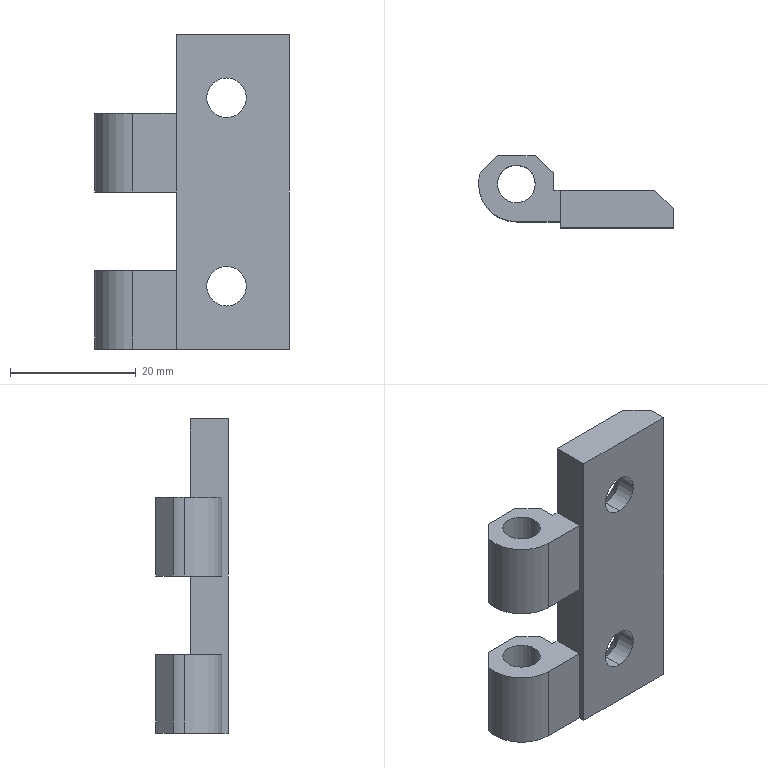Part | SolidWorks | 1 solid | 36 faces | box 31 x 11.5 x 50 mm | volume 6739 mm3 | plane 20 | cylinder 12 | cone 4 | commonest cylinder face diameters 6 x4 6.3 x4 12 x4
STEP:
#1=CARTESIAN_POINT('',(8.,3.15,-18.15));
#2=VERTEX_POINT('',#1);
#3=CARTESIAN_POINT('',(8.,3.15,-11.85));
#4=VERTEX_POINT('',#3);
#5=CARTESIAN_POINT('',(8.,3.15,-15.));
#6=DIRECTION('',(0.,1.,0.));
#7=DIRECTION('',(0.,0.,1.));
#8=AXIS2_PLACEMENT_3D('',#5,#6,#7);
#9=CIRCLE('',#8,3.15);
#10=EDGE_CURVE('',#2,#4,#9,.T.);
#11=ORIENTED_EDGE('',*,*,#10,.F.);
#12=CARTESIAN_POINT('',(8.,6.,-21.));
#13=VERTEX_POINT('',#12);
#14=CARTESIAN_POINT('',(8.,6.,-21.));
#15=DIRECTION('',(0.,0.7071,-0.7071));
#16=VECTOR('',#15,1000.);
#17=LINE('',#14,#16);
#18=EDGE_CURVE('',#2,#13,#17,.T.);
#19=ORIENTED_EDGE('',*,*,#18,.T.);
#20=CARTESIAN_POINT('',(8.,6.,-9.));
#21=VERTEX_POINT('',#20);
#22=CARTESIAN_POINT('',(8.,6.,-15.));
#23=DIRECTION('',(0.,1.,0.));
#24=DIRECTION('',(0.,0.,1.));
#25=AXIS2_PLACEMENT_3D('',#22,#23,#24);
#26=CIRCLE('',#25,6.);
#27=EDGE_CURVE('',#13,#21,#26,.T.);
#28=ORIENTED_EDGE('',*,*,#27,.T.);
#29=CARTESIAN_POINT('',(8.,6.,-9.));
#30=DIRECTION('',(0.,0.7071,0.7071));
#31=VECTOR('',#30,1000.);
#32=LINE('',#29,#31);
#33=EDGE_CURVE('',#4,#21,#32,.T.);
#34=ORIENTED_EDGE('',*,*,#33,.F.);
#35=EDGE_LOOP('',(#11,#19,#28,#34));
#36=FACE_OUTER_BOUND('',#35,.T.);
#37=CARTESIAN_POINT('',(8.,6.,-15.));
#38=DIRECTION('',(0.,1.,0.));
#39=DIRECTION('',(0.,0.,1.));
#40=AXIS2_PLACEMENT_3D('',#37,#38,#39);
#41=CONICAL_SURFACE('',#40,6.,0.7854);
#42=ADVANCED_FACE('',(#36),#41,.F.);
#43=CARTESIAN_POINT('',(8.,0.,-18.15));
#44=VERTEX_POINT('',#43);
#45=CARTESIAN_POINT('',(8.,0.,-11.85));
#46=VERTEX_POINT('',#45);
#47=CARTESIAN_POINT('',(8.,0.,-15.));
#48=DIRECTION('',(0.,1.,0.));
#49=DIRECTION('',(0.,0.,1.));
#50=AXIS2_PLACEMENT_3D('',#47,#48,#49);
#51=CIRCLE('',#50,3.15);
#52=EDGE_CURVE('',#44,#46,#51,.T.);
#53=ORIENTED_EDGE('',*,*,#52,.F.);
#54=CARTESIAN_POINT('',(8.,6.,-18.15));
#55=DIRECTION('',(0.,1.,0.));
#56=VECTOR('',#55,1000.);
#57=LINE('',#54,#56);
#58=EDGE_CURVE('',#44,#2,#57,.T.);
#59=ORIENTED_EDGE('',*,*,#58,.T.);
#60=ORIENTED_EDGE('',*,*,#10,.T.);
#61=CARTESIAN_POINT('',(8.,6.,-11.85));
#62=DIRECTION('',(0.,1.,0.));
#63=VECTOR('',#62,1000.);
#64=LINE('',#61,#63);
#65=EDGE_CURVE('',#46,#4,#64,.T.);
#66=ORIENTED_EDGE('',*,*,#65,.F.);
#67=EDGE_LOOP('',(#53,#59,#60,#66));
#68=FACE_OUTER_BOUND('',#67,.T.);
#69=CARTESIAN_POINT('',(8.,6.,-15.));
#70=DIRECTION('',(0.,1.,0.));
#71=DIRECTION('',(0.,0.,1.));
#72=AXIS2_PLACEMENT_3D('',#69,#70,#71);
#73=CYLINDRICAL_SURFACE('',#72,3.15);
#74=ADVANCED_FACE('',(#68),#73,.F.);
#75=CARTESIAN_POINT('',(8.,3.15,11.85));
#76=VERTEX_POINT('',#75);
#77=CARTESIAN_POINT('',(8.,3.15,18.15));
#78=VERTEX_POINT('',#77);
#79=CARTESIAN_POINT('',(8.,3.15,15.));
#80=DIRECTION('',(0.,1.,0.));
#81=DIRECTION('',(0.,0.,1.));
#82=AXIS2_PLACEMENT_3D('',#79,#80,#81);
#83=CIRCLE('',#82,3.15);
#84=EDGE_CURVE('',#76,#78,#83,.T.);
#85=ORIENTED_EDGE('',*,*,#84,.F.);
#86=CARTESIAN_POINT('',(8.,6.,9.));
#87=VERTEX_POINT('',#86);
#88=CARTESIAN_POINT('',(8.,6.,9.));
#89=DIRECTION('',(0.,0.7071,-0.7071));
#90=VECTOR('',#89,1000.);
#91=LINE('',#88,#90);
#92=EDGE_CURVE('',#76,#87,#91,.T.);
#93=ORIENTED_EDGE('',*,*,#92,.T.);
#94=CARTESIAN_POINT('',(8.,6.,21.));
#95=VERTEX_POINT('',#94);
#96=CARTESIAN_POINT('',(8.,6.,15.));
#97=DIRECTION('',(0.,1.,0.));
#98=DIRECTION('',(0.,0.,1.));
#99=AXIS2_PLACEMENT_3D('',#96,#97,#98);
#100=CIRCLE('',#99,6.);
#101=EDGE_CURVE('',#87,#95,#100,.T.);
#102=ORIENTED_EDGE('',*,*,#101,.T.);
#103=CARTESIAN_POINT('',(8.,6.,21.));
#104=DIRECTION('',(0.,0.7071,0.7071));
#105=VECTOR('',#104,1000.);
#106=LINE('',#103,#105);
#107=EDGE_CURVE('',#78,#95,#106,.T.);
#108=ORIENTED_EDGE('',*,*,#107,.F.);
#109=EDGE_LOOP('',(#85,#93,#102,#108));
#110=FACE_OUTER_BOUND('',#109,.T.);
#111=CARTESIAN_POINT('',(8.,6.,15.));
#112=DIRECTION('',(0.,1.,0.));
#113=DIRECTION('',(0.,0.,1.));
#114=AXIS2_PLACEMENT_3D('',#111,#112,#113);
#115=CONICAL_SURFACE('',#114,6.,0.7854);
#116=ADVANCED_FACE('',(#110),#115,.F.);
#117=CARTESIAN_POINT('',(8.,0.,11.85));
#118=VERTEX_POINT('',#117);
#119=CARTESIAN_POINT('',(8.,0.,18.15));
#120=VERTEX_POINT('',#119);
#121=CARTESIAN_POINT('',(8.,0.,15.));
#122=DIRECTION('',(0.,1.,0.));
#123=DIRECTION('',(0.,0.,1.));
#124=AXIS2_PLACEMENT_3D('',#121,#122,#123);
#125=CIRCLE('',#124,3.15);
#126=EDGE_CURVE('',#118,#120,#125,.T.);
#127=ORIENTED_EDGE('',*,*,#126,.F.);
#128=CARTESIAN_POINT('',(8.,6.,11.85));
#129=DIRECTION('',(0.,1.,0.));
#130=VECTOR('',#129,1000.);
#131=LINE('',#128,#130);
#132=EDGE_CURVE('',#118,#76,#131,.T.);
#133=ORIENTED_EDGE('',*,*,#132,.T.);
#134=ORIENTED_EDGE('',*,*,#84,.T.);
#135=CARTESIAN_POINT('',(8.,6.,18.15));
#136=DIRECTION('',(0.,1.,0.));
#137=VECTOR('',#136,1000.);
#138=LINE('',#135,#137);
#139=EDGE_CURVE('',#120,#78,#138,.T.);
#140=ORIENTED_EDGE('',*,*,#139,.F.);
#141=EDGE_LOOP('',(#127,#133,#134,#140));
#142=FACE_OUTER_BOUND('',#141,.T.);
#143=CARTESIAN_POINT('',(8.,6.,15.));
#144=DIRECTION('',(0.,1.,0.));
#145=DIRECTION('',(0.,0.,1.));
#146=AXIS2_PLACEMENT_3D('',#143,#144,#145);
#147=CYLINDRICAL_SURFACE('',#146,3.15);
#148=ADVANCED_FACE('',(#142),#147,.F.);
#149=CARTESIAN_POINT('',(-4.,7.,12.5));
#150=VERTEX_POINT('',#149);
#151=CARTESIAN_POINT('',(-10.,7.,12.5));
#152=VERTEX_POINT('',#151);
#153=CARTESIAN_POINT('',(-7.,7.,12.5));
#154=DIRECTION('',(0.,0.,-1.));
#155=DIRECTION('',(-1.,0.,0.));
#156=AXIS2_PLACEMENT_3D('',#153,#154,#155);
#157=CIRCLE('',#156,3.);
#158=EDGE_CURVE('',#150,#152,#157,.T.);
#159=ORIENTED_EDGE('',*,*,#158,.F.);
#160=CARTESIAN_POINT('',(-4.,7.,0.));
#161=VERTEX_POINT('',#160);
#162=CARTESIAN_POINT('',(-4.,7.,25.));
#163=DIRECTION('',(0.,0.,-1.));
#164=VECTOR('',#163,1000.);
#165=LINE('',#162,#164);
#166=EDGE_CURVE('',#150,#161,#165,.T.);
#167=ORIENTED_EDGE('',*,*,#166,.T.);
#168=CARTESIAN_POINT('',(-10.,7.,0.));
#169=VERTEX_POINT('',#168);
#170=CARTESIAN_POINT('',(-7.,7.,0.));
#171=DIRECTION('',(0.,0.,1.));
#172=DIRECTION('',(1.,0.,0.));
#173=AXIS2_PLACEMENT_3D('',#170,#171,#172);
#174=CIRCLE('',#173,3.);
#175=EDGE_CURVE('',#169,#161,#174,.T.);
#176=ORIENTED_EDGE('',*,*,#175,.F.);
#177=CARTESIAN_POINT('',(-10.,7.,25.));
#178=DIRECTION('',(0.,0.,-1.));
#179=VECTOR('',#178,1000.);
#180=LINE('',#177,#179);
#181=EDGE_CURVE('',#152,#169,#180,.T.);
#182=ORIENTED_EDGE('',*,*,#181,.F.);
#183=EDGE_LOOP('',(#159,#167,#176,#182));
#184=FACE_OUTER_BOUND('',#183,.T.);
#185=CARTESIAN_POINT('',(-7.,7.,25.));
#186=DIRECTION('',(0.,0.,-1.));
#187=DIRECTION('',(-1.,0.,0.));
#188=AXIS2_PLACEMENT_3D('',#185,#186,#187);
#189=CYLINDRICAL_SURFACE('',#188,3.);
#190=ADVANCED_FACE('',(#184),#189,.F.);
#191=CARTESIAN_POINT('',(-7.,1.,12.5));
#192=VERTEX_POINT('',#191);
#193=CARTESIAN_POINT('',(-13.,7.,12.5));
#194=VERTEX_POINT('',#193);
#195=CARTESIAN_POINT('',(-7.,7.,12.5));
#196=DIRECTION('',(0.,0.,-1.));
#197=DIRECTION('',(-1.,0.,0.));
#198=AXIS2_PLACEMENT_3D('',#195,#196,#197);
#199=CIRCLE('',#198,6.);
#200=EDGE_CURVE('',#192,#194,#199,.T.);
#201=ORIENTED_EDGE('',*,*,#200,.T.);
#202=CARTESIAN_POINT('',(-13.,7.,0.));
#203=VERTEX_POINT('',#202);
#204=CARTESIAN_POINT('',(-13.,7.,25.));
#205=DIRECTION('',(0.,0.,-1.));
#206=VECTOR('',#205,1000.);
#207=LINE('',#204,#206);
#208=EDGE_CURVE('',#194,#203,#207,.T.);
#209=ORIENTED_EDGE('',*,*,#208,.T.);
#210=CARTESIAN_POINT('',(-7.,1.,0.));
#211=VERTEX_POINT('',#210);
#212=CARTESIAN_POINT('',(-7.,7.,0.));
#213=DIRECTION('',(0.,0.,1.));
#214=DIRECTION('',(1.,0.,0.));
#215=AXIS2_PLACEMENT_3D('',#212,#213,#214);
#216=CIRCLE('',#215,6.);
#217=EDGE_CURVE('',#203,#211,#216,.T.);
#218=ORIENTED_EDGE('',*,*,#217,.T.);
#219=CARTESIAN_POINT('',(-7.,1.,25.));
#220=DIRECTION('',(0.,0.,-1.));
#221=VECTOR('',#220,1000.);
#222=LINE('',#219,#221);
#223=EDGE_CURVE('',#192,#211,#222,.T.);
#224=ORIENTED_EDGE('',*,*,#223,.F.);
#225=EDGE_LOOP('',(#201,#209,#218,#224));
#226=FACE_OUTER_BOUND('',#225,.T.);
#227=CARTESIAN_POINT('',(-7.,7.,25.));
#228=DIRECTION('',(0.,0.,-1.));
#229=DIRECTION('',(-1.,0.,0.));
#230=AXIS2_PLACEMENT_3D('',#227,#228,#229);
#231=CYLINDRICAL_SURFACE('',#230,6.);
#232=ADVANCED_FACE('',(#226),#231,.T.);
#233=CARTESIAN_POINT('',(-4.,7.,-12.5));
#234=VERTEX_POINT('',#233);
#235=CARTESIAN_POINT('',(-10.,7.,-12.5));
#236=VERTEX_POINT('',#235);
#237=CARTESIAN_POINT('',(-7.,7.,-12.5));
#238=DIRECTION('',(0.,0.,-1.));
#239=DIRECTION('',(-1.,0.,0.));
#240=AXIS2_PLACEMENT_3D('',#237,#238,#239);
#241=CIRCLE('',#240,3.);
#242=EDGE_CURVE('',#234,#236,#241,.T.);
#243=ORIENTED_EDGE('',*,*,#242,.F.);
#244=CARTESIAN_POINT('',(-4.,7.,-25.));
#245=VERTEX_POINT('',#244);
#246=CARTESIAN_POINT('',(-4.,7.,25.));
#247=DIRECTION('',(0.,0.,-1.));
#248=VECTOR('',#247,1000.);
#249=LINE('',#246,#248);
#250=EDGE_CURVE('',#234,#245,#249,.T.);
#251=ORIENTED_EDGE('',*,*,#250,.T.);
#252=CARTESIAN_POINT('',(-10.,7.,-25.));
#253=VERTEX_POINT('',#252);
#254=CARTESIAN_POINT('',(-7.,7.,-25.));
#255=DIRECTION('',(0.,0.,1.));
#256=DIRECTION('',(1.,0.,0.));
#257=AXIS2_PLACEMENT_3D('',#254,#255,#256);
#258=CIRCLE('',#257,3.);
#259=EDGE_CURVE('',#253,#245,#258,.T.);
#260=ORIENTED_EDGE('',*,*,#259,.F.);
#261=CARTESIAN_POINT('',(-10.,7.,25.));
#262=DIRECTION('',(0.,0.,-1.));
#263=VECTOR('',#262,1000.);
#264=LINE('',#261,#263);
#265=EDGE_CURVE('',#236,#253,#264,.T.);
#266=ORIENTED_EDGE('',*,*,#265,.F.);
#267=EDGE_LOOP('',(#243,#251,#260,#266));
#268=FACE_OUTER_BOUND('',#267,.T.);
#269=CARTESIAN_POINT('',(-7.,7.,25.));
#270=DIRECTION('',(0.,0.,-1.));
#271=DIRECTION('',(-1.,0.,0.));
#272=AXIS2_PLACEMENT_3D('',#269,#270,#271);
#273=CYLINDRICAL_SURFACE('',#272,3.);
#274=ADVANCED_FACE('',(#268),#273,.F.);
#275=CARTESIAN_POINT('',(-7.,1.,-12.5));
#276=VERTEX_POINT('',#275);
#277=CARTESIAN_POINT('',(-13.,7.,-12.5));
#278=VERTEX_POINT('',#277);
#279=CARTESIAN_POINT('',(-7.,7.,-12.5));
#280=DIRECTION('',(0.,0.,-1.));
#281=DIRECTION('',(-1.,0.,0.));
#282=AXIS2_PLACEMENT_3D('',#279,#280,#281);
#283=CIRCLE('',#282,6.);
#284=EDGE_CURVE('',#276,#278,#283,.T.);
#285=ORIENTED_EDGE('',*,*,#284,.T.);
#286=CARTESIAN_POINT('',(-13.,7.,-25.));
#287=VERTEX_POINT('',#286);
#288=CARTESIAN_POINT('',(-13.,7.,25.));
#289=DIRECTION('',(0.,0.,-1.));
#290=VECTOR('',#289,1000.);
#291=LINE('',#288,#290);
#292=EDGE_CURVE('',#278,#287,#291,.T.);
#293=ORIENTED_EDGE('',*,*,#292,.T.);
#294=CARTESIAN_POINT('',(-7.,1.,-25.));
#295=VERTEX_POINT('',#294);
#296=CARTESIAN_POINT('',(-7.,7.,-25.));
#297=DIRECTION('',(0.,0.,1.));
#298=DIRECTION('',(1.,0.,0.));
#299=AXIS2_PLACEMENT_3D('',#296,#297,#298);
#300=CIRCLE('',#299,6.);
#301=EDGE_CURVE('',#287,#295,#300,.T.);
#302=ORIENTED_EDGE('',*,*,#301,.T.);
#303=CARTESIAN_POINT('',(-7.,1.,25.));
#304=DIRECTION('',(0.,0.,-1.));
#305=VECTOR('',#304,1000.);
#306=LINE('',#303,#305);
#307=EDGE_CURVE('',#276,#295,#306,.T.);
#308=ORIENTED_EDGE('',*,*,#307,.F.);
#309=EDGE_LOOP('',(#285,#293,#302,#308));
#310=FACE_OUTER_BOUND('',#309,.T.);
#311=CARTESIAN_POINT('',(-7.,7.,25.));
#312=DIRECTION('',(0.,0.,-1.));
#313=DIRECTION('',(-1.,0.,0.));
#314=AXIS2_PLACEMENT_3D('',#311,#312,#313);
#315=CYLINDRICAL_SURFACE('',#314,6.);
#316=ADVANCED_FACE('',(#310),#315,.T.);
#317=CARTESIAN_POINT('',(-10.,11.5,-12.5));
#318=VERTEX_POINT('',#317);
#319=CARTESIAN_POINT('',(-12.74,8.748,-12.5));
#320=VERTEX_POINT('',#319);
#321=CARTESIAN_POINT('',(-10.772,10.725,-12.5));
#322=DIRECTION('',(-0.7056,-0.7087,0.));
#323=VECTOR('',#322,1000.);
#324=LINE('',#321,#323);
#325=EDGE_CURVE('',#318,#320,#324,.T.);
#326=ORIENTED_EDGE('',*,*,#325,.F.);
#327=CARTESIAN_POINT('',(-10.,11.5,-25.));
#328=VERTEX_POINT('',#327);
#329=CARTESIAN_POINT('',(-10.,11.5,25.));
#330=DIRECTION('',(0.,0.,-1.));
#331=VECTOR('',#330,1000.);
#332=LINE('',#329,#331);
#333=EDGE_CURVE('',#318,#328,#332,.T.);
#334=ORIENTED_EDGE('',*,*,#333,.T.);
#335=CARTESIAN_POINT('',(-12.74,8.748,-25.));
#336=VERTEX_POINT('',#335);
#337=CARTESIAN_POINT('',(-10.772,10.725,-25.));
#338=DIRECTION('',(0.7056,0.7087,0.));
#339=VECTOR('',#338,1000.);
#340=LINE('',#337,#339);
#341=EDGE_CURVE('',#336,#328,#340,.T.);
#342=ORIENTED_EDGE('',*,*,#341,.F.);
#343=CARTESIAN_POINT('',(-12.74,8.748,25.));
#344=DIRECTION('',(0.,0.,-1.));
#345=VECTOR('',#344,1000.);
#346=LINE('',#343,#345);
#347=EDGE_CURVE('',#320,#336,#346,.T.);
#348=ORIENTED_EDGE('',*,*,#347,.F.);
#349=EDGE_LOOP('',(#326,#334,#342,#348));
#350=FACE_OUTER_BOUND('',#349,.T.);
#351=CARTESIAN_POINT('',(-10.772,10.725,25.));
#352=DIRECTION('',(-0.7087,0.7056,0.));
#353=DIRECTION('',(-0.7056,-0.7087,0.));
#354=AXIS2_PLACEMENT_3D('',#351,#352,#353);
#355=PLANE('',#354);
#356=ADVANCED_FACE('',(#350),#355,.T.);
#357=ORIENTED_EDGE('',*,*,#292,.F.);
#358=CARTESIAN_POINT('',(-7.,7.,-12.5));
#359=DIRECTION('',(0.,0.,-1.));
#360=DIRECTION('',(-1.,0.,0.));
#361=AXIS2_PLACEMENT_3D('',#358,#359,#360);
#362=CIRCLE('',#361,6.);
#363=EDGE_CURVE('',#278,#320,#362,.T.);
#364=ORIENTED_EDGE('',*,*,#363,.T.);
#365=ORIENTED_EDGE('',*,*,#347,.T.);
#366=CARTESIAN_POINT('',(-7.,7.,-25.));
#367=DIRECTION('',(0.,0.,1.));
#368=DIRECTION('',(1.,0.,0.));
#369=AXIS2_PLACEMENT_3D('',#366,#367,#368);
#370=CIRCLE('',#369,6.);
#371=EDGE_CURVE('',#336,#287,#370,.T.);
#372=ORIENTED_EDGE('',*,*,#371,.T.);
#373=EDGE_LOOP('',(#357,#364,#365,#372));
#374=FACE_OUTER_BOUND('',#373,.T.);
#375=CARTESIAN_POINT('',(-7.,7.,25.));
#376=DIRECTION('',(0.,0.,-1.));
#377=DIRECTION('',(-1.,0.,0.));
#378=AXIS2_PLACEMENT_3D('',#375,#376,#377);
#379=CYLINDRICAL_SURFACE('',#378,6.);
#380=ADVANCED_FACE('',(#374),#379,.T.);
#381=CARTESIAN_POINT('',(0.,1.,-12.5));
#382=VERTEX_POINT('',#381);
#383=CARTESIAN_POINT('',(0.,1.,-25.));
#384=VERTEX_POINT('',#383);
#385=CARTESIAN_POINT('',(0.,1.,25.));
#386=DIRECTION('',(0.,0.,-1.));
#387=VECTOR('',#386,1000.);
#388=LINE('',#385,#387);
#389=EDGE_CURVE('',#382,#384,#388,.T.);
#390=ORIENTED_EDGE('',*,*,#389,.F.);
#391=CARTESIAN_POINT('',(0.,1.,-12.5));
#392=DIRECTION('',(-1.,0.,0.));
#393=VECTOR('',#392,1000.);
#394=LINE('',#391,#393);
#395=EDGE_CURVE('',#382,#276,#394,.T.);
#396=ORIENTED_EDGE('',*,*,#395,.T.);
#397=ORIENTED_EDGE('',*,*,#307,.T.);
#398=CARTESIAN_POINT('',(0.,1.,-25.));
#399=DIRECTION('',(1.,0.,0.));
#400=VECTOR('',#399,1000.);
#401=LINE('',#398,#400);
#402=EDGE_CURVE('',#295,#384,#401,.T.);
#403=ORIENTED_EDGE('',*,*,#402,.T.);
#404=EDGE_LOOP('',(#390,#396,#397,#403));
#405=FACE_OUTER_BOUND('',#404,.T.);
#406=CARTESIAN_POINT('',(0.,1.,25.));
#407=DIRECTION('',(0.,1.,0.));
#408=DIRECTION('',(0.,0.,1.));
#409=AXIS2_PLACEMENT_3D('',#406,#407,#408);
#410=PLANE('',#409);
#411=ADVANCED_FACE('',(#405),#410,.F.);
#412=CARTESIAN_POINT('',(-1.084,8.748,-12.5));
#413=VERTEX_POINT('',#412);
#414=CARTESIAN_POINT('',(-1.084,8.748,-25.));
#415=VERTEX_POINT('',#414);
#416=CARTESIAN_POINT('',(-1.084,8.748,25.));
#417=DIRECTION('',(0.,0.,-1.));
#418=VECTOR('',#417,1000.);
#419=LINE('',#416,#418);
#420=EDGE_CURVE('',#413,#415,#419,.T.);
#421=ORIENTED_EDGE('',*,*,#420,.F.);
#422=CARTESIAN_POINT('',(-1.084,6.,-12.5));
#423=VERTEX_POINT('',#422);
#424=CARTESIAN_POINT('',(-1.084,0.,-12.5));
#425=DIRECTION('',(0.,-1.,0.));
#426=VECTOR('',#425,1000.);
#427=LINE('',#424,#426);
#428=EDGE_CURVE('',#413,#423,#427,.T.);
#429=ORIENTED_EDGE('',*,*,#428,.T.);
#430=CARTESIAN_POINT('',(-1.084,6.,-25.));
#431=VERTEX_POINT('',#430);
#432=CARTESIAN_POINT('',(-1.084,6.,25.));
#433=DIRECTION('',(0.,0.,-1.));
#434=VECTOR('',#433,1000.);
#435=LINE('',#432,#434);
#436=EDGE_CURVE('',#423,#431,#435,.T.);
#437=ORIENTED_EDGE('',*,*,#436,.T.);
#438=CARTESIAN_POINT('',(-1.084,0.,-25.));
#439=DIRECTION('',(0.,1.,0.));
#440=VECTOR('',#439,1000.);
#441=LINE('',#438,#440);
#442=EDGE_CURVE('',#431,#415,#441,.T.);
#443=ORIENTED_EDGE('',*,*,#442,.T.);
#444=EDGE_LOOP('',(#421,#429,#437,#443));
#445=FACE_OUTER_BOUND('',#444,.T.);
#446=CARTESIAN_POINT('',(-1.084,0.,25.));
#447=DIRECTION('',(-1.,0.,0.));
#448=DIRECTION('',(0.,-1.,0.));
#449=AXIS2_PLACEMENT_3D('',#446,#447,#448);
#450=PLANE('',#449);
#451=ADVANCED_FACE('',(#445),#450,.F.);
#452=CARTESIAN_POINT('',(-4.,11.5,-12.5));
#453=VERTEX_POINT('',#452);
#454=CARTESIAN_POINT('',(-4.,11.5,-25.));
#455=VERTEX_POINT('',#454);
#456=CARTESIAN_POINT('',(-4.,11.5,25.));
#457=DIRECTION('',(0.,0.,-1.));
#458=VECTOR('',#457,1000.);
#459=LINE('',#456,#458);
#460=EDGE_CURVE('',#453,#455,#459,.T.);
#461=ORIENTED_EDGE('',*,*,#460,.F.);
#462=CARTESIAN_POINT('',(3.856,4.087,-12.5));
#463=DIRECTION('',(0.7273,-0.6863,0.));
#464=VECTOR('',#463,1000.);
#465=LINE('',#462,#464);
#466=EDGE_CURVE('',#453,#413,#465,.T.);
#467=ORIENTED_EDGE('',*,*,#466,.T.);
#468=ORIENTED_EDGE('',*,*,#420,.T.);
#469=CARTESIAN_POINT('',(3.856,4.087,-25.));
#470=DIRECTION('',(-0.7273,0.6863,0.));
#471=VECTOR('',#470,1000.);
#472=LINE('',#469,#471);
#473=EDGE_CURVE('',#415,#455,#472,.T.);
#474=ORIENTED_EDGE('',*,*,#473,.T.);
#475=EDGE_LOOP('',(#461,#467,#468,#474));
#476=FACE_OUTER_BOUND('',#475,.T.);
#477=CARTESIAN_POINT('',(3.856,4.087,25.));
#478=DIRECTION('',(-0.6863,-0.7273,0.));
#479=DIRECTION('',(0.7273,-0.6863,0.));
#480=AXIS2_PLACEMENT_3D('',#477,#478,#479);
#481=PLANE('',#480);
#482=ADVANCED_FACE('',(#476),#481,.F.);
#483=ORIENTED_EDGE('',*,*,#250,.F.);
#484=CARTESIAN_POINT('',(-7.,7.,-12.5));
#485=DIRECTION('',(0.,0.,-1.));
#486=DIRECTION('',(-1.,0.,0.));
#487=AXIS2_PLACEMENT_3D('',#484,#485,#486);
#488=CIRCLE('',#487,3.);
#489=EDGE_CURVE('',#236,#234,#488,.T.);
#490=ORIENTED_EDGE('',*,*,#489,.F.);
#491=ORIENTED_EDGE('',*,*,#265,.T.);
#492=CARTESIAN_POINT('',(-7.,7.,-25.));
#493=DIRECTION('',(0.,0.,1.));
#494=DIRECTION('',(1.,0.,0.));
#495=AXIS2_PLACEMENT_3D('',#492,#493,#494);
#496=CIRCLE('',#495,3.);
#497=EDGE_CURVE('',#245,#253,#496,.T.);
#498=ORIENTED_EDGE('',*,*,#497,.F.);
#499=EDGE_LOOP('',(#483,#490,#491,#498));
#500=FACE_OUTER_BOUND('',#499,.T.);
#501=CARTESIAN_POINT('',(-7.,7.,25.));
#502=DIRECTION('',(0.,0.,-1.));
#503=DIRECTION('',(-1.,0.,0.));
#504=AXIS2_PLACEMENT_3D('',#501,#502,#503);
#505=CYLINDRICAL_SURFACE('',#504,3.);
#506=ADVANCED_FACE('',(#500),#505,.F.);
#507=CARTESIAN_POINT('',(0.,11.5,-12.5));
#508=DIRECTION('',(-1.,0.,0.));
#509=VECTOR('',#508,1000.);
#510=LINE('',#507,#509);
#511=EDGE_CURVE('',#453,#318,#510,.T.);
#512=ORIENTED_EDGE('',*,*,#511,.F.);
#513=ORIENTED_EDGE('',*,*,#460,.T.);
#514=CARTESIAN_POINT('',(0.,11.5,-25.));
#515=DIRECTION('',(1.,0.,0.));
#516=VECTOR('',#515,1000.);
#517=LINE('',#514,#516);
#518=EDGE_CURVE('',#328,#455,#517,.T.);
#519=ORIENTED_EDGE('',*,*,#518,.F.);
#520=ORIENTED_EDGE('',*,*,#333,.F.);
#521=EDGE_LOOP('',(#512,#513,#519,#520));
#522=FACE_OUTER_BOUND('',#521,.T.);
#523=CARTESIAN_POINT('',(0.,11.5,25.));
#524=DIRECTION('',(0.,1.,0.));
#525=DIRECTION('',(-1.,0.,0.));
#526=AXIS2_PLACEMENT_3D('',#523,#524,#525);
#527=PLANE('',#526);
#528=ADVANCED_FACE('',(#522),#527,.T.);
#529=CARTESIAN_POINT('',(-10.,11.5,12.5));
#530=VERTEX_POINT('',#529);
#531=CARTESIAN_POINT('',(-12.74,8.748,12.5));
#532=VERTEX_POINT('',#531);
#533=CARTESIAN_POINT('',(-10.772,10.725,12.5));
#534=DIRECTION('',(-0.7056,-0.7087,0.));
#535=VECTOR('',#534,1000.);
#536=LINE('',#533,#535);
#537=EDGE_CURVE('',#530,#532,#536,.T.);
#538=ORIENTED_EDGE('',*,*,#537,.F.);
#539=CARTESIAN_POINT('',(-10.,11.5,0.));
#540=VERTEX_POINT('',#539);
#541=CARTESIAN_POINT('',(-10.,11.5,25.));
#542=DIRECTION('',(0.,0.,-1.));
#543=VECTOR('',#542,1000.);
#544=LINE('',#541,#543);
#545=EDGE_CURVE('',#530,#540,#544,.T.);
#546=ORIENTED_EDGE('',*,*,#545,.T.);
#547=CARTESIAN_POINT('',(-12.74,8.748,0.));
#548=VERTEX_POINT('',#547);
#549=CARTESIAN_POINT('',(-10.772,10.725,0.));
#550=DIRECTION('',(0.7056,0.7087,0.));
#551=VECTOR('',#550,1000.);
#552=LINE('',#549,#551);
#553=EDGE_CURVE('',#548,#540,#552,.T.);
#554=ORIENTED_EDGE('',*,*,#553,.F.);
#555=CARTESIAN_POINT('',(-12.74,8.748,25.));
#556=DIRECTION('',(0.,0.,-1.));
#557=VECTOR('',#556,1000.);
#558=LINE('',#555,#557);
#559=EDGE_CURVE('',#532,#548,#558,.T.);
#560=ORIENTED_EDGE('',*,*,#559,.F.);
#561=EDGE_LOOP('',(#538,#546,#554,#560));
#562=FACE_OUTER_BOUND('',#561,.T.);
#563=CARTESIAN_POINT('',(-10.772,10.725,25.));
#564=DIRECTION('',(-0.7087,0.7056,0.));
#565=DIRECTION('',(-0.7056,-0.7087,0.));
#566=AXIS2_PLACEMENT_3D('',#563,#564,#565);
#567=PLANE('',#566);
#568=ADVANCED_FACE('',(#562),#567,.T.);
#569=ORIENTED_EDGE('',*,*,#208,.F.);
#570=CARTESIAN_POINT('',(-7.,7.,12.5));
#571=DIRECTION('',(0.,0.,-1.));
#572=DIRECTION('',(-1.,0.,0.));
#573=AXIS2_PLACEMENT_3D('',#570,#571,#572);
#574=CIRCLE('',#573,6.);
#575=EDGE_CURVE('',#194,#532,#574,.T.);
#576=ORIENTED_EDGE('',*,*,#575,.T.);
#577=ORIENTED_EDGE('',*,*,#559,.T.);
#578=CARTESIAN_POINT('',(-7.,7.,0.));
#579=DIRECTION('',(0.,0.,1.));
#580=DIRECTION('',(1.,0.,0.));
#581=AXIS2_PLACEMENT_3D('',#578,#579,#580);
#582=CIRCLE('',#581,6.);
#583=EDGE_CURVE('',#548,#203,#582,.T.);
#584=ORIENTED_EDGE('',*,*,#583,.T.);
#585=EDGE_LOOP('',(#569,#576,#577,#584));
#586=FACE_OUTER_BOUND('',#585,.T.);
#587=CARTESIAN_POINT('',(-7.,7.,25.));
#588=DIRECTION('',(0.,0.,-1.));
#589=DIRECTION('',(-1.,0.,0.));
#590=AXIS2_PLACEMENT_3D('',#587,#588,#589);
#591=CYLINDRICAL_SURFACE('',#590,6.);
#592=ADVANCED_FACE('',(#586),#591,.T.);
#593=CARTESIAN_POINT('',(0.,1.,12.5));
#594=VERTEX_POINT('',#593);
#595=CARTESIAN_POINT('',(0.,1.,0.));
#596=VERTEX_POINT('',#595);
#597=CARTESIAN_POINT('',(0.,1.,25.));
#598=DIRECTION('',(0.,0.,-1.));
#599=VECTOR('',#598,1000.);
#600=LINE('',#597,#599);
#601=EDGE_CURVE('',#594,#596,#600,.T.);
#602=ORIENTED_EDGE('',*,*,#601,.F.);
#603=CARTESIAN_POINT('',(0.,1.,12.5));
#604=DIRECTION('',(-1.,0.,0.));
#605=VECTOR('',#604,1000.);
#606=LINE('',#603,#605);
#607=EDGE_CURVE('',#594,#192,#606,.T.);
#608=ORIENTED_EDGE('',*,*,#607,.T.);
#609=ORIENTED_EDGE('',*,*,#223,.T.);
#610=CARTESIAN_POINT('',(0.,1.,0.));
#611=DIRECTION('',(1.,0.,0.));
#612=VECTOR('',#611,1000.);
#613=LINE('',#610,#612);
#614=EDGE_CURVE('',#211,#596,#613,.T.);
#615=ORIENTED_EDGE('',*,*,#614,.T.);
#616=EDGE_LOOP('',(#602,#608,#609,#615));
#617=FACE_OUTER_BOUND('',#616,.T.);
#618=CARTESIAN_POINT('',(0.,1.,25.));
#619=DIRECTION('',(0.,1.,0.));
#620=DIRECTION('',(0.,0.,1.));
#621=AXIS2_PLACEMENT_3D('',#618,#619,#620);
#622=PLANE('',#621);
#623=ADVANCED_FACE('',(#617),#622,.F.);
#624=CARTESIAN_POINT('',(0.,0.,-25.));
#625=VERTEX_POINT('',#624);
#626=CARTESIAN_POINT('',(0.,0.,-25.));
#627=DIRECTION('',(0.,1.,0.));
#628=VECTOR('',#627,1000.);
#629=LINE('',#626,#628);
#630=EDGE_CURVE('',#625,#384,#629,.T.);
#631=ORIENTED_EDGE('',*,*,#630,.F.);
#632=CARTESIAN_POINT('',(0.,0.,25.));
#633=VERTEX_POINT('',#632);
#634=CARTESIAN_POINT('',(0.,0.,25.));
#635=DIRECTION('',(0.,0.,-1.));
#636=VECTOR('',#635,1000.);
#637=LINE('',#634,#636);
#638=EDGE_CURVE('',#633,#625,#637,.T.);
#639=ORIENTED_EDGE('',*,*,#638,.F.);
#640=CARTESIAN_POINT('',(0.,6.,25.));
#641=VERTEX_POINT('',#640);
#642=CARTESIAN_POINT('',(0.,0.,25.));
#643=DIRECTION('',(0.,1.,0.));
#644=VECTOR('',#643,1000.);
#645=LINE('',#642,#644);
#646=EDGE_CURVE('',#633,#641,#645,.T.);
#647=ORIENTED_EDGE('',*,*,#646,.T.);
#648=CARTESIAN_POINT('',(0.,6.,12.5));
#649=VERTEX_POINT('',#648);
#650=CARTESIAN_POINT('',(0.,6.,25.));
#651=DIRECTION('',(0.,0.,-1.));
#652=VECTOR('',#651,1000.);
#653=LINE('',#650,#652);
#654=EDGE_CURVE('',#641,#649,#653,.T.);
#655=ORIENTED_EDGE('',*,*,#654,.T.);
#656=CARTESIAN_POINT('',(0.,-38.5,12.5));
#657=DIRECTION('',(0.,1.,0.));
#658=VECTOR('',#657,1000.);
#659=LINE('',#656,#658);
#660=EDGE_CURVE('',#594,#649,#659,.T.);
#661=ORIENTED_EDGE('',*,*,#660,.F.);
#662=ORIENTED_EDGE('',*,*,#601,.T.);
#663=CARTESIAN_POINT('',(0.,6.,0.));
#664=VERTEX_POINT('',#663);
#665=CARTESIAN_POINT('',(0.,-38.5,0.));
#666=DIRECTION('',(0.,1.,0.));
#667=VECTOR('',#666,1000.);
#668=LINE('',#665,#667);
#669=EDGE_CURVE('',#596,#664,#668,.T.);
#670=ORIENTED_EDGE('',*,*,#669,.T.);
#671=CARTESIAN_POINT('',(0.,6.,-12.5));
#672=VERTEX_POINT('',#671);
#673=CARTESIAN_POINT('',(0.,6.,25.));
#674=DIRECTION('',(0.,0.,-1.));
#675=VECTOR('',#674,1000.);
#676=LINE('',#673,#675);
#677=EDGE_CURVE('',#664,#672,#676,.T.);
#678=ORIENTED_EDGE('',*,*,#677,.T.);
#679=CARTESIAN_POINT('',(0.,-38.5,-12.5));
#680=DIRECTION('',(0.,1.,0.));
#681=VECTOR('',#680,1000.);
#682=LINE('',#679,#681);
#683=EDGE_CURVE('',#382,#672,#682,.T.);
#684=ORIENTED_EDGE('',*,*,#683,.F.);
#685=ORIENTED_EDGE('',*,*,#389,.T.);
#686=EDGE_LOOP('',(#631,#639,#647,#655,#661,#662,#670,#678,#684,#685));
#687=FACE_OUTER_BOUND('',#686,.T.);
#688=CARTESIAN_POINT('',(0.,0.,25.));
#689=DIRECTION('',(-1.,0.,0.));
#690=DIRECTION('',(0.,0.,1.));
#691=AXIS2_PLACEMENT_3D('',#688,#689,#690);
#692=PLANE('',#691);
#693=ADVANCED_FACE('',(#687),#692,.T.);
#694=CARTESIAN_POINT('',(8.,0.,-15.));
#695=DIRECTION('',(0.,1.,0.));
#696=DIRECTION('',(0.,0.,1.));
#697=AXIS2_PLACEMENT_3D('',#694,#695,#696);
#698=CIRCLE('',#697,3.15);
#699=EDGE_CURVE('',#46,#44,#698,.T.);
#700=ORIENTED_EDGE('',*,*,#699,.T.);
#701=ORIENTED_EDGE('',*,*,#52,.T.);
#702=EDGE_LOOP('',(#700,#701));
#703=FACE_BOUND('',#702,.T.);
#704=CARTESIAN_POINT('',(8.,0.,15.));
#705=DIRECTION('',(0.,1.,0.));
#706=DIRECTION('',(0.,0.,1.));
#707=AXIS2_PLACEMENT_3D('',#704,#705,#706);
#708=CIRCLE('',#707,3.15);
#709=EDGE_CURVE('',#120,#118,#708,.T.);
#710=ORIENTED_EDGE('',*,*,#709,.T.);
#711=ORIENTED_EDGE('',*,*,#126,.T.);
#712=EDGE_LOOP('',(#710,#711));
#713=FACE_BOUND('',#712,.T.);
#714=CARTESIAN_POINT('',(18.,0.,-25.));
#715=VERTEX_POINT('',#714);
#716=CARTESIAN_POINT('',(0.,0.,-25.));
#717=DIRECTION('',(1.,0.,0.));
#718=VECTOR('',#717,1000.);
#719=LINE('',#716,#718);
#720=EDGE_CURVE('',#625,#715,#719,.T.);
#721=ORIENTED_EDGE('',*,*,#720,.T.);
#722=CARTESIAN_POINT('',(18.,0.,25.));
#723=VERTEX_POINT('',#722);
#724=CARTESIAN_POINT('',(18.,0.,25.));
#725=DIRECTION('',(0.,0.,-1.));
#726=VECTOR('',#725,1000.);
#727=LINE('',#724,#726);
#728=EDGE_CURVE('',#723,#715,#727,.T.);
#729=ORIENTED_EDGE('',*,*,#728,.F.);
#730=CARTESIAN_POINT('',(0.,0.,25.));
#731=DIRECTION('',(1.,0.,0.));
#732=VECTOR('',#731,1000.);
#733=LINE('',#730,#732);
#734=EDGE_CURVE('',#633,#723,#733,.T.);
#735=ORIENTED_EDGE('',*,*,#734,.F.);
#736=ORIENTED_EDGE('',*,*,#638,.T.);
#737=EDGE_LOOP('',(#721,#729,#735,#736));
#738=FACE_OUTER_BOUND('',#737,.T.);
#739=CARTESIAN_POINT('',(0.,0.,25.));
#740=DIRECTION('',(0.,1.,0.));
#741=DIRECTION('',(0.,0.,1.));
#742=AXIS2_PLACEMENT_3D('',#739,#740,#741);
#743=PLANE('',#742);
#744=ADVANCED_FACE('',(#703,#713,#738),#743,.F.);
#745=CARTESIAN_POINT('',(18.,3.,-25.));
#746=VERTEX_POINT('',#745);
#747=CARTESIAN_POINT('',(18.,0.,-25.));
#748=DIRECTION('',(0.,1.,0.));
#749=VECTOR('',#748,1000.);
#750=LINE('',#747,#749);
#751=EDGE_CURVE('',#715,#746,#750,.T.);
#752=ORIENTED_EDGE('',*,*,#751,.T.);
#753=CARTESIAN_POINT('',(18.,3.,25.));
#754=VERTEX_POINT('',#753);
#755=CARTESIAN_POINT('',(18.,3.,25.));
#756=DIRECTION('',(0.,0.,1.));
#757=VECTOR('',#756,1000.);
#758=LINE('',#755,#757);
#759=EDGE_CURVE('',#746,#754,#758,.T.);
#760=ORIENTED_EDGE('',*,*,#759,.T.);
#761=CARTESIAN_POINT('',(18.,0.,25.));
#762=DIRECTION('',(0.,1.,0.));
#763=VECTOR('',#762,1000.);
#764=LINE('',#761,#763);
#765=EDGE_CURVE('',#723,#754,#764,.T.);
#766=ORIENTED_EDGE('',*,*,#765,.F.);
#767=ORIENTED_EDGE('',*,*,#728,.T.);
#768=EDGE_LOOP('',(#752,#760,#766,#767));
#769=FACE_OUTER_BOUND('',#768,.T.);
#770=CARTESIAN_POINT('',(18.,0.,25.));
#771=DIRECTION('',(-1.,0.,0.));
#772=DIRECTION('',(0.,0.,1.));
#773=AXIS2_PLACEMENT_3D('',#770,#771,#772);
#774=PLANE('',#773);
#775=ADVANCED_FACE('',(#769),#774,.F.);
#776=CARTESIAN_POINT('',(-1.084,6.,12.5));
#777=VERTEX_POINT('',#776);
#778=CARTESIAN_POINT('',(0.,6.,12.5));
#779=DIRECTION('',(-1.,0.,0.));
#780=VECTOR('',#779,1000.);
#781=LINE('',#778,#780);
#782=EDGE_CURVE('',#649,#777,#781,.T.);
#783=ORIENTED_EDGE('',*,*,#782,.F.);
#784=ORIENTED_EDGE('',*,*,#654,.F.);
#785=CARTESIAN_POINT('',(15.,6.,25.));
#786=VERTEX_POINT('',#785);
#787=CARTESIAN_POINT('',(0.,6.,25.));
#788=DIRECTION('',(1.,0.,0.));
#789=VECTOR('',#788,1000.);
#790=LINE('',#787,#789);
#791=EDGE_CURVE('',#641,#786,#790,.T.);
#792=ORIENTED_EDGE('',*,*,#791,.T.);
#793=CARTESIAN_POINT('',(15.,6.,-25.));
#794=VERTEX_POINT('',#793);
#795=CARTESIAN_POINT('',(15.,6.,-25.));
#796=DIRECTION('',(0.,0.,-1.));
#797=VECTOR('',#796,1000.);
#798=LINE('',#795,#797);
#799=EDGE_CURVE('',#786,#794,#798,.T.);
#800=ORIENTED_EDGE('',*,*,#799,.T.);
#801=CARTESIAN_POINT('',(0.,6.,-25.));
#802=DIRECTION('',(1.,0.,0.));
#803=VECTOR('',#802,1000.);
#804=LINE('',#801,#803);
#805=EDGE_CURVE('',#431,#794,#804,.T.);
#806=ORIENTED_EDGE('',*,*,#805,.F.);
#807=ORIENTED_EDGE('',*,*,#436,.F.);
#808=CARTESIAN_POINT('',(0.,6.,-12.5));
#809=DIRECTION('',(-1.,0.,0.));
#810=VECTOR('',#809,1000.);
#811=LINE('',#808,#810);
#812=EDGE_CURVE('',#672,#423,#811,.T.);
#813=ORIENTED_EDGE('',*,*,#812,.F.);
#814=ORIENTED_EDGE('',*,*,#677,.F.);
#815=CARTESIAN_POINT('',(-1.084,6.,0.));
#816=VERTEX_POINT('',#815);
#817=CARTESIAN_POINT('',(0.,6.,0.));
#818=DIRECTION('',(1.,0.,0.));
#819=VECTOR('',#818,1000.);
#820=LINE('',#817,#819);
#821=EDGE_CURVE('',#816,#664,#820,.T.);
#822=ORIENTED_EDGE('',*,*,#821,.F.);
#823=CARTESIAN_POINT('',(-1.084,6.,25.));
#824=DIRECTION('',(0.,0.,-1.));
#825=VECTOR('',#824,1000.);
#826=LINE('',#823,#825);
#827=EDGE_CURVE('',#777,#816,#826,.T.);
#828=ORIENTED_EDGE('',*,*,#827,.F.);
#829=EDGE_LOOP('',(#783,#784,#792,#800,#806,#807,#813,#814,#822,#828));
#830=FACE_OUTER_BOUND('',#829,.T.);
#831=CARTESIAN_POINT('',(8.,6.,-15.));
#832=DIRECTION('',(0.,1.,0.));
#833=DIRECTION('',(0.,0.,1.));
#834=AXIS2_PLACEMENT_3D('',#831,#832,#833);
#835=CIRCLE('',#834,6.);
#836=EDGE_CURVE('',#21,#13,#835,.T.);
#837=ORIENTED_EDGE('',*,*,#836,.F.);
#838=ORIENTED_EDGE('',*,*,#27,.F.);
#839=EDGE_LOOP('',(#837,#838));
#840=FACE_BOUND('',#839,.T.);
#841=CARTESIAN_POINT('',(8.,6.,15.));
#842=DIRECTION('',(0.,1.,0.));
#843=DIRECTION('',(0.,0.,1.));
#844=AXIS2_PLACEMENT_3D('',#841,#842,#843);
#845=CIRCLE('',#844,6.);
#846=EDGE_CURVE('',#95,#87,#845,.T.);
#847=ORIENTED_EDGE('',*,*,#846,.F.);
#848=ORIENTED_EDGE('',*,*,#101,.F.);
#849=EDGE_LOOP('',(#847,#848));
#850=FACE_BOUND('',#849,.T.);
#851=CARTESIAN_POINT('',(0.,6.,25.));
#852=DIRECTION('',(0.,1.,0.));
#853=DIRECTION('',(-1.,0.,0.));
#854=AXIS2_PLACEMENT_3D('',#851,#852,#853);
#855=PLANE('',#854);
#856=ADVANCED_FACE('',(#830,#840,#850),#855,.T.);
#857=CARTESIAN_POINT('',(-1.084,8.748,12.5));
#858=VERTEX_POINT('',#857);
#859=CARTESIAN_POINT('',(-1.084,8.748,0.));
#860=VERTEX_POINT('',#859);
#861=CARTESIAN_POINT('',(-1.084,8.748,25.));
#862=DIRECTION('',(0.,0.,-1.));
#863=VECTOR('',#862,1000.);
#864=LINE('',#861,#863);
#865=EDGE_CURVE('',#858,#860,#864,.T.);
#866=ORIENTED_EDGE('',*,*,#865,.F.);
#867=CARTESIAN_POINT('',(-1.084,0.,12.5));
#868=DIRECTION('',(0.,-1.,0.));
#869=VECTOR('',#868,1000.);
#870=LINE('',#867,#869);
#871=EDGE_CURVE('',#858,#777,#870,.T.);
#872=ORIENTED_EDGE('',*,*,#871,.T.);
#873=ORIENTED_EDGE('',*,*,#827,.T.);
#874=CARTESIAN_POINT('',(-1.084,0.,0.));
#875=DIRECTION('',(0.,1.,0.));
#876=VECTOR('',#875,1000.);
#877=LINE('',#874,#876);
#878=EDGE_CURVE('',#816,#860,#877,.T.);
#879=ORIENTED_EDGE('',*,*,#878,.T.);
#880=EDGE_LOOP('',(#866,#872,#873,#879));
#881=FACE_OUTER_BOUND('',#880,.T.);
#882=CARTESIAN_POINT('',(-1.084,0.,25.));
#883=DIRECTION('',(-1.,0.,0.));
#884=DIRECTION('',(0.,-1.,0.));
#885=AXIS2_PLACEMENT_3D('',#882,#883,#884);
#886=PLANE('',#885);
#887=ADVANCED_FACE('',(#881),#886,.F.);
#888=CARTESIAN_POINT('',(-4.,11.5,12.5));
#889=VERTEX_POINT('',#888);
#890=CARTESIAN_POINT('',(-4.,11.5,0.));
#891=VERTEX_POINT('',#890);
#892=CARTESIAN_POINT('',(-4.,11.5,25.));
#893=DIRECTION('',(0.,0.,-1.));
#894=VECTOR('',#893,1000.);
#895=LINE('',#892,#894);
#896=EDGE_CURVE('',#889,#891,#895,.T.);
#897=ORIENTED_EDGE('',*,*,#896,.F.);
#898=CARTESIAN_POINT('',(3.856,4.087,12.5));
#899=DIRECTION('',(0.7273,-0.6863,0.));
#900=VECTOR('',#899,1000.);
#901=LINE('',#898,#900);
#902=EDGE_CURVE('',#889,#858,#901,.T.);
#903=ORIENTED_EDGE('',*,*,#902,.T.);
#904=ORIENTED_EDGE('',*,*,#865,.T.);
#905=CARTESIAN_POINT('',(3.856,4.087,0.));
#906=DIRECTION('',(-0.7273,0.6863,0.));
#907=VECTOR('',#906,1000.);
#908=LINE('',#905,#907);
#909=EDGE_CURVE('',#860,#891,#908,.T.);
#910=ORIENTED_EDGE('',*,*,#909,.T.);
#911=EDGE_LOOP('',(#897,#903,#904,#910));
#912=FACE_OUTER_BOUND('',#911,.T.);
#913=CARTESIAN_POINT('',(3.856,4.087,25.));
#914=DIRECTION('',(-0.6863,-0.7273,0.));
#915=DIRECTION('',(0.7273,-0.6863,0.));
#916=AXIS2_PLACEMENT_3D('',#913,#914,#915);
#917=PLANE('',#916);
#918=ADVANCED_FACE('',(#912),#917,.F.);
#919=ORIENTED_EDGE('',*,*,#166,.F.);
#920=CARTESIAN_POINT('',(-7.,7.,12.5));
#921=DIRECTION('',(0.,0.,-1.));
#922=DIRECTION('',(-1.,0.,0.));
#923=AXIS2_PLACEMENT_3D('',#920,#921,#922);
#924=CIRCLE('',#923,3.);
#925=EDGE_CURVE('',#152,#150,#924,.T.);
#926=ORIENTED_EDGE('',*,*,#925,.F.);
#927=ORIENTED_EDGE('',*,*,#181,.T.);
#928=CARTESIAN_POINT('',(-7.,7.,0.));
#929=DIRECTION('',(0.,0.,1.));
#930=DIRECTION('',(1.,0.,0.));
#931=AXIS2_PLACEMENT_3D('',#928,#929,#930);
#932=CIRCLE('',#931,3.);
#933=EDGE_CURVE('',#161,#169,#932,.T.);
#934=ORIENTED_EDGE('',*,*,#933,.F.);
#935=EDGE_LOOP('',(#919,#926,#927,#934));
#936=FACE_OUTER_BOUND('',#935,.T.);
#937=CARTESIAN_POINT('',(-7.,7.,25.));
#938=DIRECTION('',(0.,0.,-1.));
#939=DIRECTION('',(-1.,0.,0.));
#940=AXIS2_PLACEMENT_3D('',#937,#938,#939);
#941=CYLINDRICAL_SURFACE('',#940,3.);
#942=ADVANCED_FACE('',(#936),#941,.F.);
#943=CARTESIAN_POINT('',(-26.911,11.5,12.5));
#944=DIRECTION('',(-1.,0.,0.));
#945=VECTOR('',#944,1000.);
#946=LINE('',#943,#945);
#947=EDGE_CURVE('',#889,#530,#946,.T.);
#948=ORIENTED_EDGE('',*,*,#947,.F.);
#949=ORIENTED_EDGE('',*,*,#896,.T.);
#950=CARTESIAN_POINT('',(0.,11.5,0.));
#951=DIRECTION('',(1.,0.,0.));
#952=VECTOR('',#951,1000.);
#953=LINE('',#950,#952);
#954=EDGE_CURVE('',#540,#891,#953,.T.);
#955=ORIENTED_EDGE('',*,*,#954,.F.);
#956=ORIENTED_EDGE('',*,*,#545,.F.);
#957=EDGE_LOOP('',(#948,#949,#955,#956));
#958=FACE_OUTER_BOUND('',#957,.T.);
#959=CARTESIAN_POINT('',(0.,11.5,25.));
#960=DIRECTION('',(0.,1.,0.));
#961=DIRECTION('',(-1.,0.,0.));
#962=AXIS2_PLACEMENT_3D('',#959,#960,#961);
#963=PLANE('',#962);
#964=ADVANCED_FACE('',(#958),#963,.T.);
#965=ORIENTED_EDGE('',*,*,#791,.F.);
#966=ORIENTED_EDGE('',*,*,#646,.F.);
#967=ORIENTED_EDGE('',*,*,#734,.T.);
#968=ORIENTED_EDGE('',*,*,#765,.T.);
#969=CARTESIAN_POINT('',(10.5,10.5,25.));
#970=DIRECTION('',(-0.7071,0.7071,0.));
#971=VECTOR('',#970,1000.);
#972=LINE('',#969,#971);
#973=EDGE_CURVE('',#754,#786,#972,.T.);
#974=ORIENTED_EDGE('',*,*,#973,.T.);
#975=EDGE_LOOP('',(#965,#966,#967,#968,#974));
#976=FACE_OUTER_BOUND('',#975,.T.);
#977=CARTESIAN_POINT('',(0.,0.,25.));
#978=DIRECTION('',(0.,0.,1.));
#979=DIRECTION('',(1.,0.,0.));
#980=AXIS2_PLACEMENT_3D('',#977,#978,#979);
#981=PLANE('',#980);
#982=ADVANCED_FACE('',(#976),#981,.T.);
#983=ORIENTED_EDGE('',*,*,#259,.T.);
#984=ORIENTED_EDGE('',*,*,#497,.T.);
#985=EDGE_LOOP('',(#983,#984));
#986=FACE_BOUND('',#985,.T.);
#987=ORIENTED_EDGE('',*,*,#805,.T.);
#988=CARTESIAN_POINT('',(15.,6.,-25.));
#989=DIRECTION('',(0.7071,-0.7071,0.));
#990=VECTOR('',#989,1000.);
#991=LINE('',#988,#990);
#992=EDGE_CURVE('',#794,#746,#991,.T.);
#993=ORIENTED_EDGE('',*,*,#992,.T.);
#994=ORIENTED_EDGE('',*,*,#751,.F.);
#995=ORIENTED_EDGE('',*,*,#720,.F.);
#996=ORIENTED_EDGE('',*,*,#630,.T.);
#997=ORIENTED_EDGE('',*,*,#402,.F.);
#998=ORIENTED_EDGE('',*,*,#301,.F.);
#999=ORIENTED_EDGE('',*,*,#371,.F.);
#1000=ORIENTED_EDGE('',*,*,#341,.T.);
#1001=ORIENTED_EDGE('',*,*,#518,.T.);
#1002=ORIENTED_EDGE('',*,*,#473,.F.);
#1003=ORIENTED_EDGE('',*,*,#442,.F.);
#1004=EDGE_LOOP('',(#987,#993,#994,#995,#996,#997,#998,#999,#1000,#1001,#1002,#1003));
#1005=FACE_OUTER_BOUND('',#1004,.T.);
#1006=CARTESIAN_POINT('',(0.,0.,-25.));
#1007=DIRECTION('',(0.,0.,1.));
#1008=DIRECTION('',(1.,0.,0.));
#1009=AXIS2_PLACEMENT_3D('',#1006,#1007,#1008);
#1010=PLANE('',#1009);
#1011=ADVANCED_FACE('',(#986,#1005),#1010,.F.);
#1012=ORIENTED_EDGE('',*,*,#973,.F.);
#1013=ORIENTED_EDGE('',*,*,#759,.F.);
#1014=ORIENTED_EDGE('',*,*,#992,.F.);
#1015=ORIENTED_EDGE('',*,*,#799,.F.);
#1016=EDGE_LOOP('',(#1012,#1013,#1014,#1015));
#1017=FACE_OUTER_BOUND('',#1016,.T.);
#1018=CARTESIAN_POINT('',(15.,6.,25.));
#1019=DIRECTION('',(0.7071,0.7071,0.));
#1020=DIRECTION('',(-0.7071,0.7071,0.));
#1021=AXIS2_PLACEMENT_3D('',#1018,#1019,#1020);
#1022=PLANE('',#1021);
#1023=ADVANCED_FACE('',(#1017),#1022,.T.);
#1024=ORIENTED_EDGE('',*,*,#132,.F.);
#1025=ORIENTED_EDGE('',*,*,#709,.F.);
#1026=ORIENTED_EDGE('',*,*,#139,.T.);
#1027=CARTESIAN_POINT('',(8.,3.15,15.));
#1028=DIRECTION('',(0.,1.,0.));
#1029=DIRECTION('',(0.,0.,1.));
#1030=AXIS2_PLACEMENT_3D('',#1027,#1028,#1029);
#1031=CIRCLE('',#1030,3.15);
#1032=EDGE_CURVE('',#78,#76,#1031,.T.);
#1033=ORIENTED_EDGE('',*,*,#1032,.T.);
#1034=EDGE_LOOP('',(#1024,#1025,#1026,#1033));
#1035=FACE_OUTER_BOUND('',#1034,.T.);
#1036=CARTESIAN_POINT('',(8.,6.,15.));
#1037=DIRECTION('',(0.,1.,0.));
#1038=DIRECTION('',(0.,0.,1.));
#1039=AXIS2_PLACEMENT_3D('',#1036,#1037,#1038);
#1040=CYLINDRICAL_SURFACE('',#1039,3.15);
#1041=ADVANCED_FACE('',(#1035),#1040,.F.);
#1042=ORIENTED_EDGE('',*,*,#92,.F.);
#1043=ORIENTED_EDGE('',*,*,#1032,.F.);
#1044=ORIENTED_EDGE('',*,*,#107,.T.);
#1045=ORIENTED_EDGE('',*,*,#846,.T.);
#1046=EDGE_LOOP('',(#1042,#1043,#1044,#1045));
#1047=FACE_OUTER_BOUND('',#1046,.T.);
#1048=CARTESIAN_POINT('',(8.,6.,15.));
#1049=DIRECTION('',(0.,1.,0.));
#1050=DIRECTION('',(0.,0.,1.));
#1051=AXIS2_PLACEMENT_3D('',#1048,#1049,#1050);
#1052=CONICAL_SURFACE('',#1051,6.,0.7854);
#1053=ADVANCED_FACE('',(#1047),#1052,.F.);
#1054=ORIENTED_EDGE('',*,*,#58,.F.);
#1055=ORIENTED_EDGE('',*,*,#699,.F.);
#1056=ORIENTED_EDGE('',*,*,#65,.T.);
#1057=CARTESIAN_POINT('',(8.,3.15,-15.));
#1058=DIRECTION('',(0.,1.,0.));
#1059=DIRECTION('',(0.,0.,1.));
#1060=AXIS2_PLACEMENT_3D('',#1057,#1058,#1059);
#1061=CIRCLE('',#1060,3.15);
#1062=EDGE_CURVE('',#4,#2,#1061,.T.);
#1063=ORIENTED_EDGE('',*,*,#1062,.T.);
#1064=EDGE_LOOP('',(#1054,#1055,#1056,#1063));
#1065=FACE_OUTER_BOUND('',#1064,.T.);
#1066=CARTESIAN_POINT('',(8.,6.,-15.));
#1067=DIRECTION('',(0.,1.,0.));
#1068=DIRECTION('',(0.,0.,1.));
#1069=AXIS2_PLACEMENT_3D('',#1066,#1067,#1068);
#1070=CYLINDRICAL_SURFACE('',#1069,3.15);
#1071=ADVANCED_FACE('',(#1065),#1070,.F.);
#1072=ORIENTED_EDGE('',*,*,#18,.F.);
#1073=ORIENTED_EDGE('',*,*,#1062,.F.);
#1074=ORIENTED_EDGE('',*,*,#33,.T.);
#1075=ORIENTED_EDGE('',*,*,#836,.T.);
#1076=EDGE_LOOP('',(#1072,#1073,#1074,#1075));
#1077=FACE_OUTER_BOUND('',#1076,.T.);
#1078=CARTESIAN_POINT('',(8.,6.,-15.));
#1079=DIRECTION('',(0.,1.,0.));
#1080=DIRECTION('',(0.,0.,1.));
#1081=AXIS2_PLACEMENT_3D('',#1078,#1079,#1080);
#1082=CONICAL_SURFACE('',#1081,6.,0.7854);
#1083=ADVANCED_FACE('',(#1077),#1082,.F.);
#1084=ORIENTED_EDGE('',*,*,#325,.T.);
#1085=ORIENTED_EDGE('',*,*,#363,.F.);
#1086=ORIENTED_EDGE('',*,*,#284,.F.);
#1087=ORIENTED_EDGE('',*,*,#395,.F.);
#1088=ORIENTED_EDGE('',*,*,#683,.T.);
#1089=ORIENTED_EDGE('',*,*,#812,.T.);
#1090=ORIENTED_EDGE('',*,*,#428,.F.);
#1091=ORIENTED_EDGE('',*,*,#466,.F.);
#1092=ORIENTED_EDGE('',*,*,#511,.T.);
#1093=EDGE_LOOP('',(#1084,#1085,#1086,#1087,#1088,#1089,#1090,#1091,#1092));
#1094=FACE_OUTER_BOUND('',#1093,.T.);
#1095=ORIENTED_EDGE('',*,*,#489,.T.);
#1096=ORIENTED_EDGE('',*,*,#242,.T.);
#1097=EDGE_LOOP('',(#1095,#1096));
#1098=FACE_BOUND('',#1097,.T.);
#1099=CARTESIAN_POINT('',(-23.881,-38.5,-12.5));
#1100=DIRECTION('',(0.,0.,-1.));
#1101=DIRECTION('',(-1.,0.,0.));
#1102=AXIS2_PLACEMENT_3D('',#1099,#1100,#1101);
#1103=PLANE('',#1102);
#1104=ADVANCED_FACE('',(#1094,#1098),#1103,.F.);
#1105=ORIENTED_EDGE('',*,*,#553,.T.);
#1106=ORIENTED_EDGE('',*,*,#954,.T.);
#1107=ORIENTED_EDGE('',*,*,#909,.F.);
#1108=ORIENTED_EDGE('',*,*,#878,.F.);
#1109=ORIENTED_EDGE('',*,*,#821,.T.);
#1110=ORIENTED_EDGE('',*,*,#669,.F.);
#1111=ORIENTED_EDGE('',*,*,#614,.F.);
#1112=ORIENTED_EDGE('',*,*,#217,.F.);
#1113=ORIENTED_EDGE('',*,*,#583,.F.);
#1114=EDGE_LOOP('',(#1105,#1106,#1107,#1108,#1109,#1110,#1111,#1112,#1113));
#1115=FACE_OUTER_BOUND('',#1114,.T.);
#1116=ORIENTED_EDGE('',*,*,#175,.T.);
#1117=ORIENTED_EDGE('',*,*,#933,.T.);
#1118=EDGE_LOOP('',(#1116,#1117));
#1119=FACE_BOUND('',#1118,.T.);
#1120=CARTESIAN_POINT('',(-23.881,-38.5,0.));
#1121=DIRECTION('',(0.,0.,1.));
#1122=DIRECTION('',(1.,0.,0.));
#1123=AXIS2_PLACEMENT_3D('',#1120,#1121,#1122);
#1124=PLANE('',#1123);
#1125=ADVANCED_FACE('',(#1115,#1119),#1124,.F.);
#1126=ORIENTED_EDGE('',*,*,#537,.T.);
#1127=ORIENTED_EDGE('',*,*,#575,.F.);
#1128=ORIENTED_EDGE('',*,*,#200,.F.);
#1129=ORIENTED_EDGE('',*,*,#607,.F.);
#1130=ORIENTED_EDGE('',*,*,#660,.T.);
#1131=ORIENTED_EDGE('',*,*,#782,.T.);
#1132=ORIENTED_EDGE('',*,*,#871,.F.);
#1133=ORIENTED_EDGE('',*,*,#902,.F.);
#1134=ORIENTED_EDGE('',*,*,#947,.T.);
#1135=EDGE_LOOP('',(#1126,#1127,#1128,#1129,#1130,#1131,#1132,#1133,#1134));
#1136=FACE_OUTER_BOUND('',#1135,.T.);
#1137=ORIENTED_EDGE('',*,*,#925,.T.);
#1138=ORIENTED_EDGE('',*,*,#158,.T.);
#1139=EDGE_LOOP('',(#1137,#1138));
#1140=FACE_BOUND('',#1139,.T.);
#1141=CARTESIAN_POINT('',(-26.911,-38.5,12.5));
#1142=DIRECTION('',(0.,0.,-1.));
#1143=DIRECTION('',(-1.,0.,0.));
#1144=AXIS2_PLACEMENT_3D('',#1141,#1142,#1143);
#1145=PLANE('',#1144);
#1146=ADVANCED_FACE('',(#1136,#1140),#1145,.F.);
#1147=CLOSED_SHELL('',(#42,#74,#116,#148,#190,#232,#274,#316,#356,#380,#411,#451,#482,#506,#528,#568,#592,#623,#693,#744,#775,#856,#887,#918,#942,#964,#982,#1011,#1023,#1041,#1053,#1071,#1083,#1104,#1125,#1146));
#1148=MANIFOLD_SOLID_BREP('',#1147);
#1149=CARTESIAN_POINT('',(0.,0.,0.));
#1150=DIRECTION('',(0.,0.,1.));
#1151=DIRECTION('',(1.,0.,0.));
#1152=AXIS2_PLACEMENT_3D('',#1149,#1150,#1151);
#1153=(LENGTH_UNIT()NAMED_UNIT(*)SI_UNIT(.MILLI.,.METRE.));
#1154=UNCERTAINTY_MEASURE_WITH_UNIT(LENGTH_MEASURE(0.00001),#1153,'','');
#1155=(NAMED_UNIT(*)PLANE_ANGLE_UNIT()SI_UNIT($,.RADIAN.));
#1156=(NAMED_UNIT(*)SI_UNIT($,.STERADIAN.)SOLID_ANGLE_UNIT());
#1157=(GEOMETRIC_REPRESENTATION_CONTEXT(3)GLOBAL_UNCERTAINTY_ASSIGNED_CONTEXT((#1154))GLOBAL_UNIT_ASSIGNED_CONTEXT((#1153,#1155,#1156))REPRESENTATION_CONTEXT('',''));
#1158=ADVANCED_BREP_SHAPE_REPRESENTATION('',(#1148,#1152),#1157);